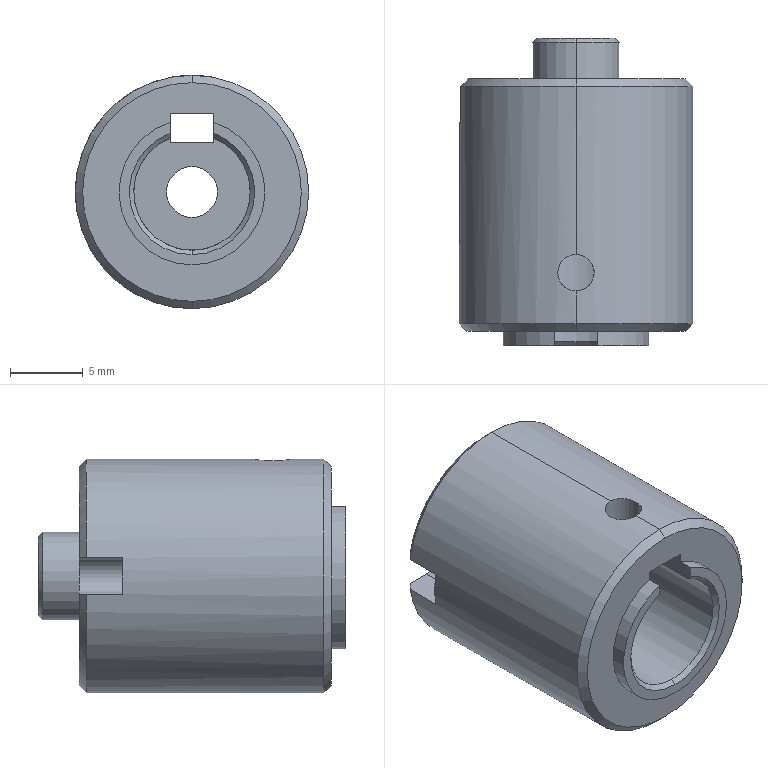Part | SolidWorks | features ICE 19, CirPattern 7, Chamfer 3, Extrusion 1, Fillet 1 | 1 solid | 35 faces | box 16 x 21.1 x 16 mm | volume 2636 mm3 | cylinder 12 | plane 12 | cone 11 | commonest cylinder face diameters 2.5 x3 3.5 x2 6 x2 10 x2 16 x2 8 x1
STEP:
#1=CARTESIAN_POINT('',(0.,4.8,2.7));
#2=VERTEX_POINT('',#1);
#3=CARTESIAN_POINT('',(0.,4.8,-2.7));
#4=VERTEX_POINT('',#3);
#5=CARTESIAN_POINT('',(0.,4.8,0.));
#6=DIRECTION('',(0.,1.,0.));
#7=DIRECTION('',(0.,0.,1.));
#8=AXIS2_PLACEMENT_3D('',#5,#6,#7);
#9=CIRCLE('',#8,2.7);
#10=EDGE_CURVE('',#2,#4,#9,.T.);
#11=ORIENTED_EDGE('',*,*,#10,.F.);
#12=CARTESIAN_POINT('',(0.,4.5,3.));
#13=VERTEX_POINT('',#12);
#14=CARTESIAN_POINT('',(0.,4.8,2.7));
#15=DIRECTION('',(0.,-0.7071,0.7071));
#16=VECTOR('',#15,1000.);
#17=LINE('',#14,#16);
#18=EDGE_CURVE('',#2,#13,#17,.T.);
#19=ORIENTED_EDGE('',*,*,#18,.T.);
#20=CARTESIAN_POINT('',(0.,4.5,-3.));
#21=VERTEX_POINT('',#20);
#22=CARTESIAN_POINT('',(0.,4.5,0.));
#23=DIRECTION('',(0.,-1.,0.));
#24=DIRECTION('',(0.,0.,1.));
#25=AXIS2_PLACEMENT_3D('',#22,#23,#24);
#26=CIRCLE('',#25,3.);
#27=EDGE_CURVE('',#21,#13,#26,.T.);
#28=ORIENTED_EDGE('',*,*,#27,.F.);
#29=CARTESIAN_POINT('',(0.,4.8,-2.7));
#30=DIRECTION('',(0.,-0.7071,-0.7071));
#31=VECTOR('',#30,1000.);
#32=LINE('',#29,#31);
#33=EDGE_CURVE('',#4,#21,#32,.T.);
#34=ORIENTED_EDGE('',*,*,#33,.F.);
#35=EDGE_LOOP('',(#11,#19,#28,#34));
#36=FACE_OUTER_BOUND('',#35,.T.);
#37=CARTESIAN_POINT('',(0.,4.8,0.));
#38=DIRECTION('',(0.,-1.,0.));
#39=DIRECTION('',(0.,0.,-1.));
#40=AXIS2_PLACEMENT_3D('',#37,#38,#39);
#41=CONICAL_SURFACE('',#40,2.7,0.7854);
#42=ADVANCED_FACE('',(#36),#41,.T.);
#43=CARTESIAN_POINT('',(0.,4.5,-1.75));
#44=VERTEX_POINT('',#43);
#45=CARTESIAN_POINT('',(0.,4.5,1.75));
#46=VERTEX_POINT('',#45);
#47=CARTESIAN_POINT('',(0.,4.5,0.));
#48=DIRECTION('',(0.,1.,0.));
#49=DIRECTION('',(0.,0.,1.));
#50=AXIS2_PLACEMENT_3D('',#47,#48,#49);
#51=CIRCLE('',#50,1.75);
#52=EDGE_CURVE('',#44,#46,#51,.T.);
#53=ORIENTED_EDGE('',*,*,#52,.F.);
#54=CARTESIAN_POINT('',(0.,4.8,-2.05));
#55=VERTEX_POINT('',#54);
#56=CARTESIAN_POINT('',(0.,4.5,-1.75));
#57=DIRECTION('',(0.,0.7071,-0.7071));
#58=VECTOR('',#57,1000.);
#59=LINE('',#56,#58);
#60=EDGE_CURVE('',#44,#55,#59,.T.);
#61=ORIENTED_EDGE('',*,*,#60,.T.);
#62=CARTESIAN_POINT('',(0.,4.8,2.05));
#63=VERTEX_POINT('',#62);
#64=CARTESIAN_POINT('',(0.,4.8,0.));
#65=DIRECTION('',(0.,-1.,0.));
#66=DIRECTION('',(0.,0.,1.));
#67=AXIS2_PLACEMENT_3D('',#64,#65,#66);
#68=CIRCLE('',#67,2.05);
#69=EDGE_CURVE('',#63,#55,#68,.T.);
#70=ORIENTED_EDGE('',*,*,#69,.F.);
#71=CARTESIAN_POINT('',(0.,4.5,1.75));
#72=DIRECTION('',(0.,0.7071,0.7071));
#73=VECTOR('',#72,1000.);
#74=LINE('',#71,#73);
#75=EDGE_CURVE('',#46,#63,#74,.T.);
#76=ORIENTED_EDGE('',*,*,#75,.F.);
#77=EDGE_LOOP('',(#53,#61,#70,#76));
#78=FACE_OUTER_BOUND('',#77,.T.);
#79=CARTESIAN_POINT('',(0.,4.5,0.));
#80=DIRECTION('',(0.,1.,0.));
#81=DIRECTION('',(0.,0.,1.));
#82=AXIS2_PLACEMENT_3D('',#79,#80,#81);
#83=CONICAL_SURFACE('',#82,1.75,0.7854);
#84=ADVANCED_FACE('',(#78),#83,.F.);
#85=CARTESIAN_POINT('',(0.,-16.,-4.));
#86=VERTEX_POINT('',#85);
#87=CARTESIAN_POINT('',(1.5,-16.,3.708));
#88=VERTEX_POINT('',#87);
#89=CARTESIAN_POINT('',(0.,-16.,0.));
#90=DIRECTION('',(0.,-1.,0.));
#91=DIRECTION('',(0.,0.,-1.));
#92=AXIS2_PLACEMENT_3D('',#89,#90,#91);
#93=CIRCLE('',#92,4.);
#94=EDGE_CURVE('',#86,#88,#93,.T.);
#95=ORIENTED_EDGE('',*,*,#94,.F.);
#96=CARTESIAN_POINT('',(0.,-16.3,-4.3));
#97=VERTEX_POINT('',#96);
#98=CARTESIAN_POINT('',(0.,-16.,-4.));
#99=DIRECTION('',(0.,-0.7071,-0.7071));
#100=VECTOR('',#99,1000.);
#101=LINE('',#98,#100);
#102=EDGE_CURVE('',#86,#97,#101,.T.);
#103=ORIENTED_EDGE('',*,*,#102,.T.);
#104=CARTESIAN_POINT('',(1.5,-16.3,4.03));
#105=VERTEX_POINT('',#104);
#106=CARTESIAN_POINT('',(0.,-16.3,0.));
#107=DIRECTION('',(0.,1.,0.));
#108=DIRECTION('',(0.,0.,-1.));
#109=AXIS2_PLACEMENT_3D('',#106,#107,#108);
#110=CIRCLE('',#109,4.3);
#111=EDGE_CURVE('',#105,#97,#110,.T.);
#112=ORIENTED_EDGE('',*,*,#111,.F.);
#113=CARTESIAN_POINT('',(1.5,-16.,3.708));
#114=CARTESIAN_POINT('',(1.5,-16.1,3.816));
#115=CARTESIAN_POINT('',(1.5,-16.2,3.923));
#116=CARTESIAN_POINT('',(1.5,-16.3,4.03));
#117=B_SPLINE_CURVE_WITH_KNOTS('',3,(#113,#114,#115,#116),.UNSPECIFIED.,.F.,.F.,(4,4),(0.,0.0004399),.UNSPECIFIED.);
#118=EDGE_CURVE('',#88,#105,#117,.T.);
#119=ORIENTED_EDGE('',*,*,#118,.F.);
#120=EDGE_LOOP('',(#95,#103,#112,#119));
#121=FACE_OUTER_BOUND('',#120,.T.);
#122=CARTESIAN_POINT('',(0.,-16.,0.));
#123=DIRECTION('',(0.,-1.,0.));
#124=DIRECTION('',(0.,0.,-1.));
#125=AXIS2_PLACEMENT_3D('',#122,#123,#124);
#126=CONICAL_SURFACE('',#125,4.,0.7854);
#127=ADVANCED_FACE('',(#121),#126,.F.);
#128=CARTESIAN_POINT('',(0.,-15.3,-7.5));
#129=VERTEX_POINT('',#128);
#130=CARTESIAN_POINT('',(0.,-15.3,7.5));
#131=VERTEX_POINT('',#130);
#132=CARTESIAN_POINT('',(0.,-15.3,0.));
#133=DIRECTION('',(0.,-1.,0.));
#134=DIRECTION('',(0.,0.,-1.));
#135=AXIS2_PLACEMENT_3D('',#132,#133,#134);
#136=CIRCLE('',#135,7.5);
#137=EDGE_CURVE('',#129,#131,#136,.T.);
#138=ORIENTED_EDGE('',*,*,#137,.F.);
#139=CARTESIAN_POINT('',(0.,-14.8,-8.));
#140=VERTEX_POINT('',#139);
#141=CARTESIAN_POINT('',(0.,-15.3,-7.5));
#142=DIRECTION('',(0.,0.7071,-0.7071));
#143=VECTOR('',#142,1000.);
#144=LINE('',#141,#143);
#145=EDGE_CURVE('',#129,#140,#144,.T.);
#146=ORIENTED_EDGE('',*,*,#145,.T.);
#147=CARTESIAN_POINT('',(0.,-14.8,8.));
#148=VERTEX_POINT('',#147);
#149=CARTESIAN_POINT('',(0.,-14.8,0.));
#150=DIRECTION('',(0.,1.,0.));
#151=DIRECTION('',(0.,0.,-1.));
#152=AXIS2_PLACEMENT_3D('',#149,#150,#151);
#153=CIRCLE('',#152,8.);
#154=EDGE_CURVE('',#148,#140,#153,.T.);
#155=ORIENTED_EDGE('',*,*,#154,.F.);
#156=CARTESIAN_POINT('',(0.,-15.3,7.5));
#157=DIRECTION('',(0.,0.7071,0.7071));
#158=VECTOR('',#157,1000.);
#159=LINE('',#156,#158);
#160=EDGE_CURVE('',#131,#148,#159,.T.);
#161=ORIENTED_EDGE('',*,*,#160,.F.);
#162=EDGE_LOOP('',(#138,#146,#155,#161));
#163=FACE_OUTER_BOUND('',#162,.T.);
#164=CARTESIAN_POINT('',(0.,-15.3,0.));
#165=DIRECTION('',(0.,1.,0.));
#166=DIRECTION('',(0.,0.,1.));
#167=AXIS2_PLACEMENT_3D('',#164,#165,#166);
#168=CONICAL_SURFACE('',#167,7.5,0.7854);
#169=ADVANCED_FACE('',(#163),#168,.T.);
#170=CARTESIAN_POINT('',(0.,2.,7.5));
#171=VERTEX_POINT('',#170);
#172=CARTESIAN_POINT('',(0.,2.,-7.5));
#173=VERTEX_POINT('',#172);
#174=CARTESIAN_POINT('',(0.,2.,0.));
#175=DIRECTION('',(0.,1.,0.));
#176=DIRECTION('',(0.,0.,1.));
#177=AXIS2_PLACEMENT_3D('',#174,#175,#176);
#178=CIRCLE('',#177,7.5);
#179=EDGE_CURVE('',#171,#173,#178,.T.);
#180=ORIENTED_EDGE('',*,*,#179,.F.);
#181=CARTESIAN_POINT('',(0.,1.5,8.));
#182=VERTEX_POINT('',#181);
#183=CARTESIAN_POINT('',(0.,2.,7.5));
#184=DIRECTION('',(0.,-0.7071,0.7071));
#185=VECTOR('',#184,1000.);
#186=LINE('',#183,#185);
#187=EDGE_CURVE('',#171,#182,#186,.T.);
#188=ORIENTED_EDGE('',*,*,#187,.T.);
#189=CARTESIAN_POINT('',(0.,1.5,-8.));
#190=VERTEX_POINT('',#189);
#191=CARTESIAN_POINT('',(0.,1.5,0.));
#192=DIRECTION('',(0.,-1.,0.));
#193=DIRECTION('',(0.,0.,1.));
#194=AXIS2_PLACEMENT_3D('',#191,#192,#193);
#195=CIRCLE('',#194,8.);
#196=EDGE_CURVE('',#190,#182,#195,.T.);
#197=ORIENTED_EDGE('',*,*,#196,.F.);
#198=CARTESIAN_POINT('',(0.,2.,-7.5));
#199=DIRECTION('',(0.,-0.7071,-0.7071));
#200=VECTOR('',#199,1000.);
#201=LINE('',#198,#200);
#202=EDGE_CURVE('',#173,#190,#201,.T.);
#203=ORIENTED_EDGE('',*,*,#202,.F.);
#204=EDGE_LOOP('',(#180,#188,#197,#203));
#205=FACE_OUTER_BOUND('',#204,.T.);
#206=CARTESIAN_POINT('',(0.,2.,0.));
#207=DIRECTION('',(0.,-1.,0.));
#208=DIRECTION('',(0.,0.,-1.));
#209=AXIS2_PLACEMENT_3D('',#206,#207,#208);
#210=CONICAL_SURFACE('',#209,7.5,0.7854);
#211=ADVANCED_FACE('',(#205),#210,.T.);
#212=CARTESIAN_POINT('',(-7.395,2.,-1.25));
#213=VERTEX_POINT('',#212);
#214=CARTESIAN_POINT('',(0.,2.,0.));
#215=DIRECTION('',(0.,1.,0.));
#216=DIRECTION('',(0.,0.,1.));
#217=AXIS2_PLACEMENT_3D('',#214,#215,#216);
#218=CIRCLE('',#217,7.5);
#219=EDGE_CURVE('',#173,#213,#218,.T.);
#220=ORIENTED_EDGE('',*,*,#219,.F.);
#221=ORIENTED_EDGE('',*,*,#202,.T.);
#222=CARTESIAN_POINT('',(-7.902,1.5,-1.25));
#223=VERTEX_POINT('',#222);
#224=CARTESIAN_POINT('',(0.,1.5,0.));
#225=DIRECTION('',(0.,-1.,0.));
#226=DIRECTION('',(0.,0.,1.));
#227=AXIS2_PLACEMENT_3D('',#224,#225,#226);
#228=CIRCLE('',#227,8.);
#229=EDGE_CURVE('',#223,#190,#228,.T.);
#230=ORIENTED_EDGE('',*,*,#229,.F.);
#231=CARTESIAN_POINT('',(-7.395,2.,-1.25));
#232=CARTESIAN_POINT('',(-7.564,1.833,-1.25));
#233=CARTESIAN_POINT('',(-7.733,1.667,-1.25));
#234=CARTESIAN_POINT('',(-7.902,1.5,-1.25));
#235=B_SPLINE_CURVE_WITH_KNOTS('',3,(#231,#232,#233,#234),.UNSPECIFIED.,.F.,.F.,(4,4),(0.,0.0007118),.UNSPECIFIED.);
#236=EDGE_CURVE('',#213,#223,#235,.T.);
#237=ORIENTED_EDGE('',*,*,#236,.F.);
#238=EDGE_LOOP('',(#220,#221,#230,#237));
#239=FACE_OUTER_BOUND('',#238,.T.);
#240=CARTESIAN_POINT('',(0.,2.,0.));
#241=DIRECTION('',(0.,-1.,0.));
#242=DIRECTION('',(0.,0.,-1.));
#243=AXIS2_PLACEMENT_3D('',#240,#241,#242);
#244=CONICAL_SURFACE('',#243,7.5,0.7854);
#245=ADVANCED_FACE('',(#239),#244,.T.);
#246=CARTESIAN_POINT('',(-1.25,-11.3,5.4));
#247=VERTEX_POINT('',#246);
#248=CARTESIAN_POINT('',(1.25,-11.3,5.4));
#249=VERTEX_POINT('',#248);
#250=CARTESIAN_POINT('',(0.,-11.3,5.4));
#251=DIRECTION('',(0.,0.,1.));
#252=DIRECTION('',(1.,0.,0.));
#253=AXIS2_PLACEMENT_3D('',#250,#251,#252);
#254=CIRCLE('',#253,1.25);
#255=EDGE_CURVE('',#247,#249,#254,.T.);
#256=ORIENTED_EDGE('',*,*,#255,.F.);
#257=CARTESIAN_POINT('',(-1.25,-11.3,7.902));
#258=VERTEX_POINT('',#257);
#259=CARTESIAN_POINT('',(-1.25,-11.3,3.));
#260=DIRECTION('',(0.,0.,1.));
#261=VECTOR('',#260,1000.);
#262=LINE('',#259,#261);
#263=EDGE_CURVE('',#247,#258,#262,.T.);
#264=ORIENTED_EDGE('',*,*,#263,.T.);
#265=CARTESIAN_POINT('',(0.,-12.55,8.));
#266=VERTEX_POINT('',#265);
#267=CARTESIAN_POINT('',(0.,-12.55,8.));
#268=CARTESIAN_POINT('',(-0.1655,-12.55,8.));
#269=CARTESIAN_POINT('',(-0.3279,-12.517,7.995));
#270=CARTESIAN_POINT('',(-0.6306,-12.392,7.977));
#271=CARTESIAN_POINT('',(-0.7691,-12.299,7.964));
#272=CARTESIAN_POINT('',(-0.9994,-12.068,7.938));
#273=CARTESIAN_POINT('',(-1.092,-11.929,7.925));
#274=CARTESIAN_POINT('',(-1.217,-11.628,7.907));
#275=CARTESIAN_POINT('',(-1.25,-11.463,7.902));
#276=CARTESIAN_POINT('',(-1.25,-11.3,7.902));
#277=B_SPLINE_CURVE_WITH_KNOTS('',3,(#267,#268,#269,#270,#271,#272,#273,#274,#275,#276),.UNSPECIFIED.,.F.,.F.,(4,2,2,2,4),(0.,0.0004894,0.0009788,0.001468,0.001958),.UNSPECIFIED.);
#278=EDGE_CURVE('',#266,#258,#277,.T.);
#279=ORIENTED_EDGE('',*,*,#278,.F.);
#280=CARTESIAN_POINT('',(1.25,-11.3,7.902));
#281=VERTEX_POINT('',#280);
#282=CARTESIAN_POINT('',(1.25,-11.3,7.902));
#283=CARTESIAN_POINT('',(1.25,-11.465,7.902));
#284=CARTESIAN_POINT('',(1.217,-11.628,7.907));
#285=CARTESIAN_POINT('',(1.092,-11.93,7.925));
#286=CARTESIAN_POINT('',(0.9992,-12.069,7.938));
#287=CARTESIAN_POINT('',(0.7692,-12.299,7.964));
#288=CARTESIAN_POINT('',(0.6301,-12.392,7.977));
#289=CARTESIAN_POINT('',(0.3296,-12.517,7.995));
#290=CARTESIAN_POINT('',(0.1653,-12.55,8.));
#291=CARTESIAN_POINT('',(0.,-12.55,8.));
#292=B_SPLINE_CURVE_WITH_KNOTS('',3,(#282,#283,#284,#285,#286,#287,#288,#289,#290,#291),.UNSPECIFIED.,.F.,.F.,(4,2,2,2,4),(0.005871,0.00636,0.006849,0.007338,0.007827),.UNSPECIFIED.);
#293=EDGE_CURVE('',#281,#266,#292,.T.);
#294=ORIENTED_EDGE('',*,*,#293,.F.);
#295=CARTESIAN_POINT('',(1.25,-11.3,3.));
#296=DIRECTION('',(0.,0.,1.));
#297=VECTOR('',#296,1000.);
#298=LINE('',#295,#297);
#299=EDGE_CURVE('',#249,#281,#298,.T.);
#300=ORIENTED_EDGE('',*,*,#299,.F.);
#301=EDGE_LOOP('',(#256,#264,#279,#294,#300));
#302=FACE_OUTER_BOUND('',#301,.T.);
#303=CARTESIAN_POINT('',(0.,-11.3,3.));
#304=DIRECTION('',(0.,0.,1.));
#305=DIRECTION('',(1.,0.,0.));
#306=AXIS2_PLACEMENT_3D('',#303,#304,#305);
#307=CYLINDRICAL_SURFACE('',#306,1.25);
#308=ADVANCED_FACE('',(#302),#307,.F.);
#309=ORIENTED_EDGE('',*,*,#27,.T.);
#310=CARTESIAN_POINT('',(0.,2.,3.));
#311=VERTEX_POINT('',#310);
#312=CARTESIAN_POINT('',(0.,4.8,3.));
#313=DIRECTION('',(0.,-1.,0.));
#314=VECTOR('',#313,1000.);
#315=LINE('',#312,#314);
#316=EDGE_CURVE('',#13,#311,#315,.T.);
#317=ORIENTED_EDGE('',*,*,#316,.T.);
#318=CARTESIAN_POINT('',(0.,2.,-3.));
#319=VERTEX_POINT('',#318);
#320=CARTESIAN_POINT('',(0.,2.,0.));
#321=DIRECTION('',(0.,1.,0.));
#322=DIRECTION('',(0.,0.,1.));
#323=AXIS2_PLACEMENT_3D('',#320,#321,#322);
#324=CIRCLE('',#323,3.);
#325=EDGE_CURVE('',#311,#319,#324,.T.);
#326=ORIENTED_EDGE('',*,*,#325,.T.);
#327=CARTESIAN_POINT('',(0.,4.8,-3.));
#328=DIRECTION('',(0.,-1.,0.));
#329=VECTOR('',#328,1000.);
#330=LINE('',#327,#329);
#331=EDGE_CURVE('',#21,#319,#330,.T.);
#332=ORIENTED_EDGE('',*,*,#331,.F.);
#333=EDGE_LOOP('',(#309,#317,#326,#332));
#334=FACE_OUTER_BOUND('',#333,.T.);
#335=CARTESIAN_POINT('',(0.,4.8,0.));
#336=DIRECTION('',(0.,-1.,0.));
#337=DIRECTION('',(0.,0.,-1.));
#338=AXIS2_PLACEMENT_3D('',#335,#336,#337);
#339=CYLINDRICAL_SURFACE('',#338,3.);
#340=ADVANCED_FACE('',(#334),#339,.T.);
#341=ORIENTED_EDGE('',*,*,#52,.T.);
#342=CARTESIAN_POINT('',(0.,0.,1.75));
#343=VERTEX_POINT('',#342);
#344=CARTESIAN_POINT('',(0.,2.,1.75));
#345=DIRECTION('',(0.,-1.,0.));
#346=VECTOR('',#345,1000.);
#347=LINE('',#344,#346);
#348=EDGE_CURVE('',#46,#343,#347,.T.);
#349=ORIENTED_EDGE('',*,*,#348,.T.);
#350=CARTESIAN_POINT('',(0.,0.,-1.75));
#351=VERTEX_POINT('',#350);
#352=CARTESIAN_POINT('',(0.,0.,0.));
#353=DIRECTION('',(0.,1.,0.));
#354=DIRECTION('',(0.,0.,1.));
#355=AXIS2_PLACEMENT_3D('',#352,#353,#354);
#356=CIRCLE('',#355,1.75);
#357=EDGE_CURVE('',#351,#343,#356,.T.);
#358=ORIENTED_EDGE('',*,*,#357,.F.);
#359=CARTESIAN_POINT('',(0.,2.,-1.75));
#360=DIRECTION('',(0.,-1.,0.));
#361=VECTOR('',#360,1000.);
#362=LINE('',#359,#361);
#363=EDGE_CURVE('',#44,#351,#362,.T.);
#364=ORIENTED_EDGE('',*,*,#363,.F.);
#365=EDGE_LOOP('',(#341,#349,#358,#364));
#366=FACE_OUTER_BOUND('',#365,.T.);
#367=CARTESIAN_POINT('',(0.,2.,0.));
#368=DIRECTION('',(0.,-1.,0.));
#369=DIRECTION('',(0.,0.,-1.));
#370=AXIS2_PLACEMENT_3D('',#367,#368,#369);
#371=CYLINDRICAL_SURFACE('',#370,1.75);
#372=ADVANCED_FACE('',(#366),#371,.F.);
#373=CARTESIAN_POINT('',(-1.5,-15.3,4.77));
#374=VERTEX_POINT('',#373);
#375=CARTESIAN_POINT('',(0.,-15.3,-5.));
#376=VERTEX_POINT('',#375);
#377=CARTESIAN_POINT('',(0.,-15.3,0.));
#378=DIRECTION('',(0.,-1.,0.));
#379=DIRECTION('',(0.,0.,-1.));
#380=AXIS2_PLACEMENT_3D('',#377,#378,#379);
#381=CIRCLE('',#380,5.);
#382=EDGE_CURVE('',#374,#376,#381,.T.);
#383=ORIENTED_EDGE('',*,*,#382,.T.);
#384=CARTESIAN_POINT('',(0.,-16.3,-5.));
#385=VERTEX_POINT('',#384);
#386=CARTESIAN_POINT('',(0.,-15.3,-5.));
#387=DIRECTION('',(0.,-1.,0.));
#388=VECTOR('',#387,1000.);
#389=LINE('',#386,#388);
#390=EDGE_CURVE('',#376,#385,#389,.T.);
#391=ORIENTED_EDGE('',*,*,#390,.T.);
#392=CARTESIAN_POINT('',(-1.5,-16.3,4.77));
#393=VERTEX_POINT('',#392);
#394=CARTESIAN_POINT('',(0.,-16.3,0.));
#395=DIRECTION('',(0.,-1.,0.));
#396=DIRECTION('',(0.,0.,-1.));
#397=AXIS2_PLACEMENT_3D('',#394,#395,#396);
#398=CIRCLE('',#397,5.);
#399=EDGE_CURVE('',#393,#385,#398,.T.);
#400=ORIENTED_EDGE('',*,*,#399,.F.);
#401=CARTESIAN_POINT('',(-1.5,-15.3,4.77));
#402=DIRECTION('',(0.,-1.,0.));
#403=VECTOR('',#402,1000.);
#404=LINE('',#401,#403);
#405=EDGE_CURVE('',#374,#393,#404,.T.);
#406=ORIENTED_EDGE('',*,*,#405,.F.);
#407=EDGE_LOOP('',(#383,#391,#400,#406));
#408=FACE_OUTER_BOUND('',#407,.T.);
#409=CARTESIAN_POINT('',(0.,-15.3,0.));
#410=DIRECTION('',(0.,-1.,0.));
#411=DIRECTION('',(0.,0.,-1.));
#412=AXIS2_PLACEMENT_3D('',#409,#410,#411);
#413=CYLINDRICAL_SURFACE('',#412,5.);
#414=ADVANCED_FACE('',(#408),#413,.T.);
#415=ORIENTED_EDGE('',*,*,#154,.T.);
#416=CARTESIAN_POINT('',(0.,-16.3,-8.));
#417=DIRECTION('',(0.,1.,0.));
#418=VECTOR('',#417,1000.);
#419=LINE('',#416,#418);
#420=EDGE_CURVE('',#140,#190,#419,.T.);
#421=ORIENTED_EDGE('',*,*,#420,.T.);
#422=ORIENTED_EDGE('',*,*,#196,.T.);
#423=CARTESIAN_POINT('',(0.,-10.05,8.));
#424=VERTEX_POINT('',#423);
#425=CARTESIAN_POINT('',(0.,-16.3,8.));
#426=DIRECTION('',(0.,1.,0.));
#427=VECTOR('',#426,1000.);
#428=LINE('',#425,#427);
#429=EDGE_CURVE('',#424,#182,#428,.T.);
#430=ORIENTED_EDGE('',*,*,#429,.F.);
#431=CARTESIAN_POINT('',(0.,-10.05,8.));
#432=CARTESIAN_POINT('',(0.1633,-10.05,8.));
#433=CARTESIAN_POINT('',(0.3281,-10.083,7.995));
#434=CARTESIAN_POINT('',(0.6291,-10.208,7.977));
#435=CARTESIAN_POINT('',(0.7683,-10.301,7.964));
#436=CARTESIAN_POINT('',(0.9412,-10.473,7.945));
#437=CARTESIAN_POINT('',(0.994,-10.538,7.938));
#438=CARTESIAN_POINT('',(1.085,-10.673,7.926));
#439=CARTESIAN_POINT('',(1.123,-10.745,7.921));
#440=CARTESIAN_POINT('',(1.217,-10.972,7.907));
#441=CARTESIAN_POINT('',(1.25,-11.135,7.902));
#442=CARTESIAN_POINT('',(1.25,-11.3,7.902));
#443=B_SPLINE_CURVE_WITH_KNOTS('',3,(#431,#432,#433,#434,#435,#436,#437,#438,#439,#440,#441,#442),.UNSPECIFIED.,.F.,.F.,(4,2,2,2,2,4),(0.003914,0.004403,0.004893,0.005137,0.005382,0.005871),.UNSPECIFIED.);
#444=EDGE_CURVE('',#424,#281,#443,.T.);
#445=ORIENTED_EDGE('',*,*,#444,.T.);
#446=ORIENTED_EDGE('',*,*,#293,.T.);
#447=CARTESIAN_POINT('',(0.,-16.3,8.));
#448=DIRECTION('',(0.,1.,0.));
#449=VECTOR('',#448,1000.);
#450=LINE('',#447,#449);
#451=EDGE_CURVE('',#148,#266,#450,.T.);
#452=ORIENTED_EDGE('',*,*,#451,.F.);
#453=EDGE_LOOP('',(#415,#421,#422,#430,#445,#446,#452));
#454=FACE_OUTER_BOUND('',#453,.T.);
#455=CARTESIAN_POINT('',(0.,-16.3,0.));
#456=DIRECTION('',(0.,1.,0.));
#457=DIRECTION('',(0.,0.,1.));
#458=AXIS2_PLACEMENT_3D('',#455,#456,#457);
#459=CYLINDRICAL_SURFACE('',#458,8.);
#460=ADVANCED_FACE('',(#454),#459,.T.);
#461=CARTESIAN_POINT('',(-1.5,2.,3.4));
#462=VERTEX_POINT('',#461);
#463=CARTESIAN_POINT('',(-1.5,2.,5.4));
#464=VERTEX_POINT('',#463);
#465=CARTESIAN_POINT('',(-1.5,2.,0.));
#466=DIRECTION('',(0.,0.,1.));
#467=VECTOR('',#466,1000.);
#468=LINE('',#465,#467);
#469=EDGE_CURVE('',#462,#464,#468,.T.);
#470=ORIENTED_EDGE('',*,*,#469,.F.);
#471=CARTESIAN_POINT('',(1.5,2.,3.4));
#472=VERTEX_POINT('',#471);
#473=CARTESIAN_POINT('',(0.,2.,3.4));
#474=DIRECTION('',(-1.,0.,0.));
#475=VECTOR('',#474,1000.);
#476=LINE('',#473,#475);
#477=EDGE_CURVE('',#472,#462,#476,.T.);
#478=ORIENTED_EDGE('',*,*,#477,.F.);
#479=CARTESIAN_POINT('',(1.5,2.,5.4));
#480=VERTEX_POINT('',#479);
#481=CARTESIAN_POINT('',(1.5,2.,0.));
#482=DIRECTION('',(0.,0.,-1.));
#483=VECTOR('',#482,1000.);
#484=LINE('',#481,#483);
#485=EDGE_CURVE('',#480,#472,#484,.T.);
#486=ORIENTED_EDGE('',*,*,#485,.F.);
#487=CARTESIAN_POINT('',(0.,2.,5.4));
#488=DIRECTION('',(1.,0.,0.));
#489=VECTOR('',#488,1000.);
#490=LINE('',#487,#489);
#491=EDGE_CURVE('',#464,#480,#490,.T.);
#492=ORIENTED_EDGE('',*,*,#491,.F.);
#493=EDGE_LOOP('',(#470,#478,#486,#492));
#494=FACE_BOUND('',#493,.T.);
#495=CARTESIAN_POINT('',(-7.395,2.,1.25));
#496=VERTEX_POINT('',#495);
#497=CARTESIAN_POINT('',(-5.8,2.,1.25));
#498=VERTEX_POINT('',#497);
#499=CARTESIAN_POINT('',(-9.,2.,1.25));
#500=DIRECTION('',(1.,0.,0.));
#501=VECTOR('',#500,1000.);
#502=LINE('',#499,#501);
#503=EDGE_CURVE('',#496,#498,#502,.T.);
#504=ORIENTED_EDGE('',*,*,#503,.F.);
#505=CARTESIAN_POINT('',(0.,2.,0.));
#506=DIRECTION('',(0.,1.,0.));
#507=DIRECTION('',(0.,0.,1.));
#508=AXIS2_PLACEMENT_3D('',#505,#506,#507);
#509=CIRCLE('',#508,7.5);
#510=EDGE_CURVE('',#496,#171,#509,.T.);
#511=ORIENTED_EDGE('',*,*,#510,.T.);
#512=ORIENTED_EDGE('',*,*,#179,.T.);
#513=ORIENTED_EDGE('',*,*,#219,.T.);
#514=CARTESIAN_POINT('',(-5.8,2.,-1.25));
#515=VERTEX_POINT('',#514);
#516=CARTESIAN_POINT('',(-9.,2.,-1.25));
#517=DIRECTION('',(-1.,0.,0.));
#518=VECTOR('',#517,1000.);
#519=LINE('',#516,#518);
#520=EDGE_CURVE('',#515,#213,#519,.T.);
#521=ORIENTED_EDGE('',*,*,#520,.F.);
#522=CARTESIAN_POINT('',(-5.8,2.,0.));
#523=DIRECTION('',(0.,1.,0.));
#524=DIRECTION('',(0.,0.,-1.));
#525=AXIS2_PLACEMENT_3D('',#522,#523,#524);
#526=CIRCLE('',#525,1.25);
#527=EDGE_CURVE('',#498,#515,#526,.T.);
#528=ORIENTED_EDGE('',*,*,#527,.F.);
#529=EDGE_LOOP('',(#504,#511,#512,#513,#521,#528));
#530=FACE_OUTER_BOUND('',#529,.T.);
#531=CARTESIAN_POINT('',(0.,2.,0.));
#532=DIRECTION('',(0.,1.,0.));
#533=DIRECTION('',(0.,0.,1.));
#534=AXIS2_PLACEMENT_3D('',#531,#532,#533);
#535=CIRCLE('',#534,3.);
#536=EDGE_CURVE('',#319,#311,#535,.T.);
#537=ORIENTED_EDGE('',*,*,#536,.F.);
#538=ORIENTED_EDGE('',*,*,#325,.F.);
#539=EDGE_LOOP('',(#537,#538));
#540=FACE_BOUND('',#539,.T.);
#541=CARTESIAN_POINT('',(0.,2.,0.));
#542=DIRECTION('',(0.,1.,0.));
#543=DIRECTION('',(0.,0.,1.));
#544=AXIS2_PLACEMENT_3D('',#541,#542,#543);
#545=PLANE('',#544);
#546=ADVANCED_FACE('',(#494,#530,#540),#545,.T.);
#547=CARTESIAN_POINT('',(1.5,-16.3,4.77));
#548=VERTEX_POINT('',#547);
#549=CARTESIAN_POINT('',(1.5,-16.3,5.4));
#550=DIRECTION('',(0.,0.,1.));
#551=VECTOR('',#550,1000.);
#552=LINE('',#549,#551);
#553=EDGE_CURVE('',#105,#548,#552,.T.);
#554=ORIENTED_EDGE('',*,*,#553,.F.);
#555=ORIENTED_EDGE('',*,*,#111,.T.);
#556=CARTESIAN_POINT('',(-1.5,-16.3,4.03));
#557=VERTEX_POINT('',#556);
#558=CARTESIAN_POINT('',(0.,-16.3,0.));
#559=DIRECTION('',(0.,1.,0.));
#560=DIRECTION('',(0.,0.,-1.));
#561=AXIS2_PLACEMENT_3D('',#558,#559,#560);
#562=CIRCLE('',#561,4.3);
#563=EDGE_CURVE('',#97,#557,#562,.T.);
#564=ORIENTED_EDGE('',*,*,#563,.T.);
#565=CARTESIAN_POINT('',(-1.5,-16.3,5.4));
#566=DIRECTION('',(0.,0.,-1.));
#567=VECTOR('',#566,1000.);
#568=LINE('',#565,#567);
#569=EDGE_CURVE('',#393,#557,#568,.T.);
#570=ORIENTED_EDGE('',*,*,#569,.F.);
#571=ORIENTED_EDGE('',*,*,#399,.T.);
#572=CARTESIAN_POINT('',(0.,-16.3,0.));
#573=DIRECTION('',(0.,-1.,0.));
#574=DIRECTION('',(0.,0.,-1.));
#575=AXIS2_PLACEMENT_3D('',#572,#573,#574);
#576=CIRCLE('',#575,5.);
#577=EDGE_CURVE('',#385,#548,#576,.T.);
#578=ORIENTED_EDGE('',*,*,#577,.T.);
#579=EDGE_LOOP('',(#554,#555,#564,#570,#571,#578));
#580=FACE_OUTER_BOUND('',#579,.T.);
#581=CARTESIAN_POINT('',(0.,-16.3,0.));
#582=DIRECTION('',(0.,-1.,0.));
#583=DIRECTION('',(0.,0.,-1.));
#584=AXIS2_PLACEMENT_3D('',#581,#582,#583);
#585=PLANE('',#584);
#586=ADVANCED_FACE('',(#580),#585,.T.);
#587=ORIENTED_EDGE('',*,*,#420,.F.);
#588=CARTESIAN_POINT('',(0.,-14.8,0.));
#589=DIRECTION('',(0.,1.,0.));
#590=DIRECTION('',(0.,0.,-1.));
#591=AXIS2_PLACEMENT_3D('',#588,#589,#590);
#592=CIRCLE('',#591,8.);
#593=EDGE_CURVE('',#140,#148,#592,.T.);
#594=ORIENTED_EDGE('',*,*,#593,.T.);
#595=ORIENTED_EDGE('',*,*,#451,.T.);
#596=ORIENTED_EDGE('',*,*,#278,.T.);
#597=CARTESIAN_POINT('',(-1.25,-11.3,7.902));
#598=CARTESIAN_POINT('',(-1.25,-11.218,7.902));
#599=CARTESIAN_POINT('',(-1.242,-11.135,7.903));
#600=CARTESIAN_POINT('',(-1.21,-10.975,7.908));
#601=CARTESIAN_POINT('',(-1.186,-10.897,7.912));
#602=CARTESIAN_POINT('',(-1.092,-10.67,7.925));
#603=CARTESIAN_POINT('',(-1.,-10.532,7.938));
#604=CARTESIAN_POINT('',(-0.7673,-10.3,7.964));
#605=CARTESIAN_POINT('',(-0.6297,-10.208,7.977));
#606=CARTESIAN_POINT('',(-0.4029,-10.114,7.99));
#607=CARTESIAN_POINT('',(-0.325,-10.09,7.994));
#608=CARTESIAN_POINT('',(-0.1645,-10.058,7.999));
#609=CARTESIAN_POINT('',(-0.08163,-10.05,8.));
#610=CARTESIAN_POINT('',(0.,-10.05,8.));
#611=B_SPLINE_CURVE_WITH_KNOTS('',3,(#597,#598,#599,#600,#601,#602,#603,#604,#605,#606,#607,#608,#609,#610),.UNSPECIFIED.,.F.,.F.,(4,2,2,2,2,2,4),(0.001958,0.002202,0.002447,0.002936,0.003425,0.003669,0.003914),.UNSPECIFIED.);
#612=EDGE_CURVE('',#258,#424,#611,.T.);
#613=ORIENTED_EDGE('',*,*,#612,.T.);
#614=ORIENTED_EDGE('',*,*,#429,.T.);
#615=CARTESIAN_POINT('',(-7.902,1.5,1.25));
#616=VERTEX_POINT('',#615);
#617=CARTESIAN_POINT('',(0.,1.5,0.));
#618=DIRECTION('',(0.,-1.,0.));
#619=DIRECTION('',(0.,0.,1.));
#620=AXIS2_PLACEMENT_3D('',#617,#618,#619);
#621=CIRCLE('',#620,8.);
#622=EDGE_CURVE('',#182,#616,#621,.T.);
#623=ORIENTED_EDGE('',*,*,#622,.T.);
#624=CARTESIAN_POINT('',(-7.902,-1.,1.25));
#625=VERTEX_POINT('',#624);
#626=CARTESIAN_POINT('',(-7.902,-16.3,1.25));
#627=DIRECTION('',(0.,-1.,0.));
#628=VECTOR('',#627,1000.);
#629=LINE('',#626,#628);
#630=EDGE_CURVE('',#616,#625,#629,.T.);
#631=ORIENTED_EDGE('',*,*,#630,.T.);
#632=CARTESIAN_POINT('',(-7.902,-1.,-1.25));
#633=VERTEX_POINT('',#632);
#634=CARTESIAN_POINT('',(0.,-1.,0.));
#635=DIRECTION('',(0.,-1.,0.));
#636=DIRECTION('',(0.,0.,-1.));
#637=AXIS2_PLACEMENT_3D('',#634,#635,#636);
#638=CIRCLE('',#637,8.);
#639=EDGE_CURVE('',#625,#633,#638,.T.);
#640=ORIENTED_EDGE('',*,*,#639,.T.);
#641=CARTESIAN_POINT('',(-7.902,-16.3,-1.25));
#642=DIRECTION('',(0.,1.,0.));
#643=VECTOR('',#642,1000.);
#644=LINE('',#641,#643);
#645=EDGE_CURVE('',#633,#223,#644,.T.);
#646=ORIENTED_EDGE('',*,*,#645,.T.);
#647=ORIENTED_EDGE('',*,*,#229,.T.);
#648=EDGE_LOOP('',(#587,#594,#595,#596,#613,#614,#623,#631,#640,#646,#647));
#649=FACE_OUTER_BOUND('',#648,.T.);
#650=CARTESIAN_POINT('',(0.,-16.3,0.));
#651=DIRECTION('',(0.,1.,0.));
#652=DIRECTION('',(0.,0.,1.));
#653=AXIS2_PLACEMENT_3D('',#650,#651,#652);
#654=CYLINDRICAL_SURFACE('',#653,8.);
#655=ADVANCED_FACE('',(#649),#654,.T.);
#656=CARTESIAN_POINT('',(-1.5,0.,3.708));
#657=VERTEX_POINT('',#656);
#658=CARTESIAN_POINT('',(-1.5,-16.,3.708));
#659=VERTEX_POINT('',#658);
#660=CARTESIAN_POINT('',(-1.5,0.,3.708));
#661=DIRECTION('',(0.,-1.,0.));
#662=VECTOR('',#661,1000.);
#663=LINE('',#660,#662);
#664=EDGE_CURVE('',#657,#659,#663,.T.);
#665=ORIENTED_EDGE('',*,*,#664,.T.);
#666=CARTESIAN_POINT('',(0.,-16.,0.));
#667=DIRECTION('',(0.,-1.,0.));
#668=DIRECTION('',(0.,0.,-1.));
#669=AXIS2_PLACEMENT_3D('',#666,#667,#668);
#670=CIRCLE('',#669,4.);
#671=EDGE_CURVE('',#659,#86,#670,.T.);
#672=ORIENTED_EDGE('',*,*,#671,.T.);
#673=ORIENTED_EDGE('',*,*,#94,.T.);
#674=CARTESIAN_POINT('',(1.5,0.,3.708));
#675=VERTEX_POINT('',#674);
#676=CARTESIAN_POINT('',(1.5,0.,3.708));
#677=DIRECTION('',(0.,1.,0.));
#678=VECTOR('',#677,1000.);
#679=LINE('',#676,#678);
#680=EDGE_CURVE('',#88,#675,#679,.T.);
#681=ORIENTED_EDGE('',*,*,#680,.T.);
#682=CARTESIAN_POINT('',(0.,0.,0.));
#683=DIRECTION('',(0.,-1.,0.));
#684=DIRECTION('',(0.,0.,1.));
#685=AXIS2_PLACEMENT_3D('',#682,#683,#684);
#686=CIRCLE('',#685,4.);
#687=EDGE_CURVE('',#657,#675,#686,.T.);
#688=ORIENTED_EDGE('',*,*,#687,.F.);
#689=EDGE_LOOP('',(#665,#672,#673,#681,#688));
#690=FACE_OUTER_BOUND('',#689,.T.);
#691=CARTESIAN_POINT('',(0.,0.,0.));
#692=DIRECTION('',(0.,1.,0.));
#693=DIRECTION('',(0.,0.,1.));
#694=AXIS2_PLACEMENT_3D('',#691,#692,#693);
#695=CYLINDRICAL_SURFACE('',#694,4.);
#696=ADVANCED_FACE('',(#690),#695,.F.);
#697=CARTESIAN_POINT('',(0.,-15.3,0.));
#698=DIRECTION('',(0.,-1.,0.));
#699=DIRECTION('',(0.,0.,-1.));
#700=AXIS2_PLACEMENT_3D('',#697,#698,#699);
#701=CIRCLE('',#700,7.5);
#702=EDGE_CURVE('',#131,#129,#701,.T.);
#703=ORIENTED_EDGE('',*,*,#702,.T.);
#704=ORIENTED_EDGE('',*,*,#137,.T.);
#705=EDGE_LOOP('',(#703,#704));
#706=FACE_OUTER_BOUND('',#705,.T.);
#707=CARTESIAN_POINT('',(1.5,-15.3,4.77));
#708=VERTEX_POINT('',#707);
#709=CARTESIAN_POINT('',(1.5,-15.3,5.4));
#710=VERTEX_POINT('',#709);
#711=CARTESIAN_POINT('',(1.5,-15.3,0.));
#712=DIRECTION('',(0.,0.,1.));
#713=VECTOR('',#712,1000.);
#714=LINE('',#711,#713);
#715=EDGE_CURVE('',#708,#710,#714,.T.);
#716=ORIENTED_EDGE('',*,*,#715,.F.);
#717=CARTESIAN_POINT('',(0.,-15.3,0.));
#718=DIRECTION('',(0.,-1.,0.));
#719=DIRECTION('',(0.,0.,-1.));
#720=AXIS2_PLACEMENT_3D('',#717,#718,#719);
#721=CIRCLE('',#720,5.);
#722=EDGE_CURVE('',#376,#708,#721,.T.);
#723=ORIENTED_EDGE('',*,*,#722,.F.);
#724=ORIENTED_EDGE('',*,*,#382,.F.);
#725=CARTESIAN_POINT('',(-1.5,-15.3,5.4));
#726=VERTEX_POINT('',#725);
#727=CARTESIAN_POINT('',(-1.5,-15.3,0.));
#728=DIRECTION('',(0.,0.,-1.));
#729=VECTOR('',#728,1000.);
#730=LINE('',#727,#729);
#731=EDGE_CURVE('',#726,#374,#730,.T.);
#732=ORIENTED_EDGE('',*,*,#731,.F.);
#733=CARTESIAN_POINT('',(0.,-15.3,5.4));
#734=DIRECTION('',(-1.,0.,0.));
#735=VECTOR('',#734,1000.);
#736=LINE('',#733,#735);
#737=EDGE_CURVE('',#710,#726,#736,.T.);
#738=ORIENTED_EDGE('',*,*,#737,.F.);
#739=EDGE_LOOP('',(#716,#723,#724,#732,#738));
#740=FACE_BOUND('',#739,.T.);
#741=CARTESIAN_POINT('',(0.,-15.3,0.));
#742=DIRECTION('',(0.,-1.,0.));
#743=DIRECTION('',(0.,0.,-1.));
#744=AXIS2_PLACEMENT_3D('',#741,#742,#743);
#745=PLANE('',#744);
#746=ADVANCED_FACE('',(#706,#740),#745,.T.);
#747=ORIENTED_EDGE('',*,*,#390,.F.);
#748=ORIENTED_EDGE('',*,*,#722,.T.);
#749=CARTESIAN_POINT('',(1.5,-15.3,4.77));
#750=DIRECTION('',(0.,1.,0.));
#751=VECTOR('',#750,1000.);
#752=LINE('',#749,#751);
#753=EDGE_CURVE('',#548,#708,#752,.T.);
#754=ORIENTED_EDGE('',*,*,#753,.F.);
#755=ORIENTED_EDGE('',*,*,#577,.F.);
#756=EDGE_LOOP('',(#747,#748,#754,#755));
#757=FACE_OUTER_BOUND('',#756,.T.);
#758=CARTESIAN_POINT('',(0.,-15.3,0.));
#759=DIRECTION('',(0.,-1.,0.));
#760=DIRECTION('',(0.,0.,-1.));
#761=AXIS2_PLACEMENT_3D('',#758,#759,#760);
#762=CYLINDRICAL_SURFACE('',#761,5.);
#763=ADVANCED_FACE('',(#757),#762,.T.);
#764=ORIENTED_EDGE('',*,*,#680,.F.);
#765=ORIENTED_EDGE('',*,*,#118,.T.);
#766=ORIENTED_EDGE('',*,*,#553,.T.);
#767=ORIENTED_EDGE('',*,*,#753,.T.);
#768=ORIENTED_EDGE('',*,*,#715,.T.);
#769=CARTESIAN_POINT('',(1.5,5.8,5.4));
#770=DIRECTION('',(0.,-1.,0.));
#771=VECTOR('',#770,1000.);
#772=LINE('',#769,#771);
#773=EDGE_CURVE('',#480,#710,#772,.T.);
#774=ORIENTED_EDGE('',*,*,#773,.F.);
#775=ORIENTED_EDGE('',*,*,#485,.T.);
#776=CARTESIAN_POINT('',(1.5,0.,3.4));
#777=VERTEX_POINT('',#776);
#778=CARTESIAN_POINT('',(1.5,4.8,3.4));
#779=DIRECTION('',(0.,-1.,0.));
#780=VECTOR('',#779,1000.);
#781=LINE('',#778,#780);
#782=EDGE_CURVE('',#472,#777,#781,.T.);
#783=ORIENTED_EDGE('',*,*,#782,.T.);
#784=CARTESIAN_POINT('',(1.5,0.,0.));
#785=DIRECTION('',(0.,0.,-1.));
#786=VECTOR('',#785,1000.);
#787=LINE('',#784,#786);
#788=EDGE_CURVE('',#675,#777,#787,.T.);
#789=ORIENTED_EDGE('',*,*,#788,.F.);
#790=EDGE_LOOP('',(#764,#765,#766,#767,#768,#774,#775,#783,#789));
#791=FACE_OUTER_BOUND('',#790,.T.);
#792=CARTESIAN_POINT('',(1.5,5.8,5.4));
#793=DIRECTION('',(1.,0.,0.));
#794=DIRECTION('',(0.,0.,-1.));
#795=AXIS2_PLACEMENT_3D('',#792,#793,#794);
#796=PLANE('',#795);
#797=ADVANCED_FACE('',(#791),#796,.F.);
#798=ORIENTED_EDGE('',*,*,#569,.T.);
#799=CARTESIAN_POINT('',(-1.5,-16.3,4.03));
#800=CARTESIAN_POINT('',(-1.5,-16.2,3.923));
#801=CARTESIAN_POINT('',(-1.5,-16.1,3.816));
#802=CARTESIAN_POINT('',(-1.5,-16.,3.708));
#803=B_SPLINE_CURVE_WITH_KNOTS('',3,(#799,#800,#801,#802),.UNSPECIFIED.,.F.,.F.,(4,4),(0.,0.0004399),.UNSPECIFIED.);
#804=EDGE_CURVE('',#557,#659,#803,.T.);
#805=ORIENTED_EDGE('',*,*,#804,.T.);
#806=ORIENTED_EDGE('',*,*,#664,.F.);
#807=CARTESIAN_POINT('',(-1.5,0.,3.4));
#808=VERTEX_POINT('',#807);
#809=CARTESIAN_POINT('',(-1.5,0.,0.));
#810=DIRECTION('',(0.,0.,1.));
#811=VECTOR('',#810,1000.);
#812=LINE('',#809,#811);
#813=EDGE_CURVE('',#808,#657,#812,.T.);
#814=ORIENTED_EDGE('',*,*,#813,.F.);
#815=CARTESIAN_POINT('',(-1.5,4.8,3.4));
#816=DIRECTION('',(0.,-1.,0.));
#817=VECTOR('',#816,1000.);
#818=LINE('',#815,#817);
#819=EDGE_CURVE('',#462,#808,#818,.T.);
#820=ORIENTED_EDGE('',*,*,#819,.F.);
#821=ORIENTED_EDGE('',*,*,#469,.T.);
#822=CARTESIAN_POINT('',(-1.5,5.8,5.4));
#823=DIRECTION('',(0.,-1.,0.));
#824=VECTOR('',#823,1000.);
#825=LINE('',#822,#824);
#826=EDGE_CURVE('',#464,#726,#825,.T.);
#827=ORIENTED_EDGE('',*,*,#826,.T.);
#828=ORIENTED_EDGE('',*,*,#731,.T.);
#829=ORIENTED_EDGE('',*,*,#405,.T.);
#830=EDGE_LOOP('',(#798,#805,#806,#814,#820,#821,#827,#828,#829));
#831=FACE_OUTER_BOUND('',#830,.T.);
#832=CARTESIAN_POINT('',(-1.5,5.8,5.4));
#833=DIRECTION('',(-1.,0.,0.));
#834=DIRECTION('',(0.,0.,1.));
#835=AXIS2_PLACEMENT_3D('',#832,#833,#834);
#836=PLANE('',#835);
#837=ADVANCED_FACE('',(#831),#836,.F.);
#838=CARTESIAN_POINT('',(0.,-11.3,5.4));
#839=DIRECTION('',(0.,0.,1.));
#840=DIRECTION('',(1.,0.,0.));
#841=AXIS2_PLACEMENT_3D('',#838,#839,#840);
#842=CIRCLE('',#841,1.25);
#843=EDGE_CURVE('',#249,#247,#842,.T.);
#844=ORIENTED_EDGE('',*,*,#843,.T.);
#845=ORIENTED_EDGE('',*,*,#255,.T.);
#846=EDGE_LOOP('',(#844,#845));
#847=FACE_BOUND('',#846,.T.);
#848=ORIENTED_EDGE('',*,*,#826,.F.);
#849=ORIENTED_EDGE('',*,*,#491,.T.);
#850=ORIENTED_EDGE('',*,*,#773,.T.);
#851=ORIENTED_EDGE('',*,*,#737,.T.);
#852=EDGE_LOOP('',(#848,#849,#850,#851));
#853=FACE_OUTER_BOUND('',#852,.T.);
#854=CARTESIAN_POINT('',(-1.5,5.8,5.4));
#855=DIRECTION('',(0.,0.,1.));
#856=DIRECTION('',(1.,0.,0.));
#857=AXIS2_PLACEMENT_3D('',#854,#855,#856);
#858=PLANE('',#857);
#859=ADVANCED_FACE('',(#847,#853),#858,.F.);
#860=ORIENTED_EDGE('',*,*,#357,.T.);
#861=CARTESIAN_POINT('',(0.,0.,0.));
#862=DIRECTION('',(0.,1.,0.));
#863=DIRECTION('',(0.,0.,1.));
#864=AXIS2_PLACEMENT_3D('',#861,#862,#863);
#865=CIRCLE('',#864,1.75);
#866=EDGE_CURVE('',#343,#351,#865,.T.);
#867=ORIENTED_EDGE('',*,*,#866,.T.);
#868=EDGE_LOOP('',(#860,#867));
#869=FACE_BOUND('',#868,.T.);
#870=CARTESIAN_POINT('',(0.,0.,3.4));
#871=DIRECTION('',(-1.,0.,0.));
#872=VECTOR('',#871,1000.);
#873=LINE('',#870,#872);
#874=EDGE_CURVE('',#777,#808,#873,.T.);
#875=ORIENTED_EDGE('',*,*,#874,.T.);
#876=ORIENTED_EDGE('',*,*,#813,.T.);
#877=ORIENTED_EDGE('',*,*,#687,.T.);
#878=ORIENTED_EDGE('',*,*,#788,.T.);
#879=EDGE_LOOP('',(#875,#876,#877,#878));
#880=FACE_OUTER_BOUND('',#879,.T.);
#881=CARTESIAN_POINT('',(0.,0.,0.));
#882=DIRECTION('',(0.,1.,0.));
#883=DIRECTION('',(0.,0.,1.));
#884=AXIS2_PLACEMENT_3D('',#881,#882,#883);
#885=PLANE('',#884);
#886=ADVANCED_FACE('',(#869,#880),#885,.F.);
#887=ORIENTED_EDGE('',*,*,#348,.F.);
#888=CARTESIAN_POINT('',(0.,4.5,0.));
#889=DIRECTION('',(0.,1.,0.));
#890=DIRECTION('',(0.,0.,1.));
#891=AXIS2_PLACEMENT_3D('',#888,#889,#890);
#892=CIRCLE('',#891,1.75);
#893=EDGE_CURVE('',#46,#44,#892,.T.);
#894=ORIENTED_EDGE('',*,*,#893,.T.);
#895=ORIENTED_EDGE('',*,*,#363,.T.);
#896=ORIENTED_EDGE('',*,*,#866,.F.);
#897=EDGE_LOOP('',(#887,#894,#895,#896));
#898=FACE_OUTER_BOUND('',#897,.T.);
#899=CARTESIAN_POINT('',(0.,2.,0.));
#900=DIRECTION('',(0.,-1.,0.));
#901=DIRECTION('',(0.,0.,-1.));
#902=AXIS2_PLACEMENT_3D('',#899,#900,#901);
#903=CYLINDRICAL_SURFACE('',#902,1.75);
#904=ADVANCED_FACE('',(#898),#903,.F.);
#905=ORIENTED_EDGE('',*,*,#69,.T.);
#906=CARTESIAN_POINT('',(0.,4.8,0.));
#907=DIRECTION('',(0.,-1.,0.));
#908=DIRECTION('',(0.,0.,1.));
#909=AXIS2_PLACEMENT_3D('',#906,#907,#908);
#910=CIRCLE('',#909,2.05);
#911=EDGE_CURVE('',#55,#63,#910,.T.);
#912=ORIENTED_EDGE('',*,*,#911,.T.);
#913=EDGE_LOOP('',(#905,#912));
#914=FACE_BOUND('',#913,.T.);
#915=CARTESIAN_POINT('',(0.,4.8,0.));
#916=DIRECTION('',(0.,1.,0.));
#917=DIRECTION('',(0.,0.,1.));
#918=AXIS2_PLACEMENT_3D('',#915,#916,#917);
#919=CIRCLE('',#918,2.7);
#920=EDGE_CURVE('',#4,#2,#919,.T.);
#921=ORIENTED_EDGE('',*,*,#920,.T.);
#922=ORIENTED_EDGE('',*,*,#10,.T.);
#923=EDGE_LOOP('',(#921,#922));
#924=FACE_OUTER_BOUND('',#923,.T.);
#925=CARTESIAN_POINT('',(0.,4.8,0.));
#926=DIRECTION('',(0.,1.,0.));
#927=DIRECTION('',(0.,0.,1.));
#928=AXIS2_PLACEMENT_3D('',#925,#926,#927);
#929=PLANE('',#928);
#930=ADVANCED_FACE('',(#914,#924),#929,.T.);
#931=ORIENTED_EDGE('',*,*,#316,.F.);
#932=CARTESIAN_POINT('',(0.,4.5,0.));
#933=DIRECTION('',(0.,-1.,0.));
#934=DIRECTION('',(0.,0.,1.));
#935=AXIS2_PLACEMENT_3D('',#932,#933,#934);
#936=CIRCLE('',#935,3.);
#937=EDGE_CURVE('',#13,#21,#936,.T.);
#938=ORIENTED_EDGE('',*,*,#937,.T.);
#939=ORIENTED_EDGE('',*,*,#331,.T.);
#940=ORIENTED_EDGE('',*,*,#536,.T.);
#941=EDGE_LOOP('',(#931,#938,#939,#940));
#942=FACE_OUTER_BOUND('',#941,.T.);
#943=CARTESIAN_POINT('',(0.,4.8,0.));
#944=DIRECTION('',(0.,-1.,0.));
#945=DIRECTION('',(0.,0.,-1.));
#946=AXIS2_PLACEMENT_3D('',#943,#944,#945);
#947=CYLINDRICAL_SURFACE('',#946,3.);
#948=ADVANCED_FACE('',(#942),#947,.T.);
#949=ORIENTED_EDGE('',*,*,#263,.F.);
#950=ORIENTED_EDGE('',*,*,#843,.F.);
#951=ORIENTED_EDGE('',*,*,#299,.T.);
#952=ORIENTED_EDGE('',*,*,#444,.F.);
#953=ORIENTED_EDGE('',*,*,#612,.F.);
#954=EDGE_LOOP('',(#949,#950,#951,#952,#953));
#955=FACE_OUTER_BOUND('',#954,.T.);
#956=CARTESIAN_POINT('',(0.,-11.3,3.));
#957=DIRECTION('',(0.,0.,1.));
#958=DIRECTION('',(1.,0.,0.));
#959=AXIS2_PLACEMENT_3D('',#956,#957,#958);
#960=CYLINDRICAL_SURFACE('',#959,1.25);
#961=ADVANCED_FACE('',(#955),#960,.F.);
#962=ORIENTED_EDGE('',*,*,#630,.F.);
#963=CARTESIAN_POINT('',(-7.902,1.5,1.25));
#964=CARTESIAN_POINT('',(-7.733,1.667,1.25));
#965=CARTESIAN_POINT('',(-7.564,1.833,1.25));
#966=CARTESIAN_POINT('',(-7.395,2.,1.25));
#967=B_SPLINE_CURVE_WITH_KNOTS('',3,(#963,#964,#965,#966),.UNSPECIFIED.,.F.,.F.,(4,4),(0.,0.0007118),.UNSPECIFIED.);
#968=EDGE_CURVE('',#616,#496,#967,.T.);
#969=ORIENTED_EDGE('',*,*,#968,.T.);
#970=ORIENTED_EDGE('',*,*,#503,.T.);
#971=CARTESIAN_POINT('',(-5.8,-1.,1.25));
#972=VERTEX_POINT('',#971);
#973=CARTESIAN_POINT('',(-5.8,-1.,1.25));
#974=DIRECTION('',(0.,1.,0.));
#975=VECTOR('',#974,1000.);
#976=LINE('',#973,#975);
#977=EDGE_CURVE('',#972,#498,#976,.T.);
#978=ORIENTED_EDGE('',*,*,#977,.F.);
#979=CARTESIAN_POINT('',(-9.,-1.,1.25));
#980=DIRECTION('',(1.,0.,0.));
#981=VECTOR('',#980,1000.);
#982=LINE('',#979,#981);
#983=EDGE_CURVE('',#625,#972,#982,.T.);
#984=ORIENTED_EDGE('',*,*,#983,.F.);
#985=EDGE_LOOP('',(#962,#969,#970,#978,#984));
#986=FACE_OUTER_BOUND('',#985,.T.);
#987=CARTESIAN_POINT('',(-9.,-1.,1.25));
#988=DIRECTION('',(0.,0.,1.));
#989=DIRECTION('',(1.,0.,0.));
#990=AXIS2_PLACEMENT_3D('',#987,#988,#989);
#991=PLANE('',#990);
#992=ADVANCED_FACE('',(#986),#991,.F.);
#993=ORIENTED_EDGE('',*,*,#520,.T.);
#994=ORIENTED_EDGE('',*,*,#236,.T.);
#995=ORIENTED_EDGE('',*,*,#645,.F.);
#996=CARTESIAN_POINT('',(-5.8,-1.,-1.25));
#997=VERTEX_POINT('',#996);
#998=CARTESIAN_POINT('',(-9.,-1.,-1.25));
#999=DIRECTION('',(-1.,0.,0.));
#1000=VECTOR('',#999,1000.);
#1001=LINE('',#998,#1000);
#1002=EDGE_CURVE('',#997,#633,#1001,.T.);
#1003=ORIENTED_EDGE('',*,*,#1002,.F.);
#1004=CARTESIAN_POINT('',(-5.8,-1.,-1.25));
#1005=DIRECTION('',(0.,1.,0.));
#1006=VECTOR('',#1005,1000.);
#1007=LINE('',#1004,#1006);
#1008=EDGE_CURVE('',#997,#515,#1007,.T.);
#1009=ORIENTED_EDGE('',*,*,#1008,.T.);
#1010=EDGE_LOOP('',(#993,#994,#995,#1003,#1009));
#1011=FACE_OUTER_BOUND('',#1010,.T.);
#1012=CARTESIAN_POINT('',(-9.,-1.,-1.25));
#1013=DIRECTION('',(0.,0.,-1.));
#1014=DIRECTION('',(-1.,0.,0.));
#1015=AXIS2_PLACEMENT_3D('',#1012,#1013,#1014);
#1016=PLANE('',#1015);
#1017=ADVANCED_FACE('',(#1011),#1016,.F.);
#1018=ORIENTED_EDGE('',*,*,#983,.T.);
#1019=CARTESIAN_POINT('',(-5.8,-1.,0.));
#1020=DIRECTION('',(0.,1.,0.));
#1021=DIRECTION('',(0.,0.,-1.));
#1022=AXIS2_PLACEMENT_3D('',#1019,#1020,#1021);
#1023=CIRCLE('',#1022,1.25);
#1024=EDGE_CURVE('',#972,#997,#1023,.T.);
#1025=ORIENTED_EDGE('',*,*,#1024,.T.);
#1026=ORIENTED_EDGE('',*,*,#1002,.T.);
#1027=ORIENTED_EDGE('',*,*,#639,.F.);
#1028=EDGE_LOOP('',(#1018,#1025,#1026,#1027));
#1029=FACE_OUTER_BOUND('',#1028,.T.);
#1030=CARTESIAN_POINT('',(-5.8,-1.,0.));
#1031=DIRECTION('',(0.,-1.,0.));
#1032=DIRECTION('',(0.,0.,-1.));
#1033=AXIS2_PLACEMENT_3D('',#1030,#1031,#1032);
#1034=PLANE('',#1033);
#1035=ADVANCED_FACE('',(#1029),#1034,.F.);
#1036=ORIENTED_EDGE('',*,*,#527,.T.);
#1037=ORIENTED_EDGE('',*,*,#1008,.F.);
#1038=ORIENTED_EDGE('',*,*,#1024,.F.);
#1039=ORIENTED_EDGE('',*,*,#977,.T.);
#1040=EDGE_LOOP('',(#1036,#1037,#1038,#1039));
#1041=FACE_OUTER_BOUND('',#1040,.T.);
#1042=CARTESIAN_POINT('',(-5.8,-1.,0.));
#1043=DIRECTION('',(0.,1.,0.));
#1044=DIRECTION('',(0.,0.,1.));
#1045=AXIS2_PLACEMENT_3D('',#1042,#1043,#1044);
#1046=CYLINDRICAL_SURFACE('',#1045,1.25);
#1047=ADVANCED_FACE('',(#1041),#1046,.F.);
#1048=ORIENTED_EDGE('',*,*,#477,.T.);
#1049=ORIENTED_EDGE('',*,*,#819,.T.);
#1050=ORIENTED_EDGE('',*,*,#874,.F.);
#1051=ORIENTED_EDGE('',*,*,#782,.F.);
#1052=EDGE_LOOP('',(#1048,#1049,#1050,#1051));
#1053=FACE_OUTER_BOUND('',#1052,.T.);
#1054=CARTESIAN_POINT('',(1.5,4.8,3.4));
#1055=DIRECTION('',(0.,0.,-1.));
#1056=DIRECTION('',(-1.,0.,0.));
#1057=AXIS2_PLACEMENT_3D('',#1054,#1055,#1056);
#1058=PLANE('',#1057);
#1059=ADVANCED_FACE('',(#1053),#1058,.F.);
#1060=ORIENTED_EDGE('',*,*,#187,.F.);
#1061=ORIENTED_EDGE('',*,*,#510,.F.);
#1062=ORIENTED_EDGE('',*,*,#968,.F.);
#1063=ORIENTED_EDGE('',*,*,#622,.F.);
#1064=EDGE_LOOP('',(#1060,#1061,#1062,#1063));
#1065=FACE_OUTER_BOUND('',#1064,.T.);
#1066=CARTESIAN_POINT('',(0.,2.,0.));
#1067=DIRECTION('',(0.,-1.,0.));
#1068=DIRECTION('',(0.,0.,-1.));
#1069=AXIS2_PLACEMENT_3D('',#1066,#1067,#1068);
#1070=CONICAL_SURFACE('',#1069,7.5,0.7854);
#1071=ADVANCED_FACE('',(#1065),#1070,.T.);
#1072=ORIENTED_EDGE('',*,*,#145,.F.);
#1073=ORIENTED_EDGE('',*,*,#702,.F.);
#1074=ORIENTED_EDGE('',*,*,#160,.T.);
#1075=ORIENTED_EDGE('',*,*,#593,.F.);
#1076=EDGE_LOOP('',(#1072,#1073,#1074,#1075));
#1077=FACE_OUTER_BOUND('',#1076,.T.);
#1078=CARTESIAN_POINT('',(0.,-15.3,0.));
#1079=DIRECTION('',(0.,1.,0.));
#1080=DIRECTION('',(0.,0.,1.));
#1081=AXIS2_PLACEMENT_3D('',#1078,#1079,#1080);
#1082=CONICAL_SURFACE('',#1081,7.5,0.7854);
#1083=ADVANCED_FACE('',(#1077),#1082,.T.);
#1084=ORIENTED_EDGE('',*,*,#102,.F.);
#1085=ORIENTED_EDGE('',*,*,#671,.F.);
#1086=ORIENTED_EDGE('',*,*,#804,.F.);
#1087=ORIENTED_EDGE('',*,*,#563,.F.);
#1088=EDGE_LOOP('',(#1084,#1085,#1086,#1087));
#1089=FACE_OUTER_BOUND('',#1088,.T.);
#1090=CARTESIAN_POINT('',(0.,-16.,0.));
#1091=DIRECTION('',(0.,-1.,0.));
#1092=DIRECTION('',(0.,0.,-1.));
#1093=AXIS2_PLACEMENT_3D('',#1090,#1091,#1092);
#1094=CONICAL_SURFACE('',#1093,4.,0.7854);
#1095=ADVANCED_FACE('',(#1089),#1094,.F.);
#1096=ORIENTED_EDGE('',*,*,#60,.F.);
#1097=ORIENTED_EDGE('',*,*,#893,.F.);
#1098=ORIENTED_EDGE('',*,*,#75,.T.);
#1099=ORIENTED_EDGE('',*,*,#911,.F.);
#1100=EDGE_LOOP('',(#1096,#1097,#1098,#1099));
#1101=FACE_OUTER_BOUND('',#1100,.T.);
#1102=CARTESIAN_POINT('',(0.,4.5,0.));
#1103=DIRECTION('',(0.,1.,0.));
#1104=DIRECTION('',(0.,0.,1.));
#1105=AXIS2_PLACEMENT_3D('',#1102,#1103,#1104);
#1106=CONICAL_SURFACE('',#1105,1.75,0.7854);
#1107=ADVANCED_FACE('',(#1101),#1106,.F.);
#1108=ORIENTED_EDGE('',*,*,#18,.F.);
#1109=ORIENTED_EDGE('',*,*,#920,.F.);
#1110=ORIENTED_EDGE('',*,*,#33,.T.);
#1111=ORIENTED_EDGE('',*,*,#937,.F.);
#1112=EDGE_LOOP('',(#1108,#1109,#1110,#1111));
#1113=FACE_OUTER_BOUND('',#1112,.T.);
#1114=CARTESIAN_POINT('',(0.,4.8,0.));
#1115=DIRECTION('',(0.,-1.,0.));
#1116=DIRECTION('',(0.,0.,-1.));
#1117=AXIS2_PLACEMENT_3D('',#1114,#1115,#1116);
#1118=CONICAL_SURFACE('',#1117,2.7,0.7854);
#1119=ADVANCED_FACE('',(#1113),#1118,.T.);
#1120=CLOSED_SHELL('',(#42,#84,#127,#169,#211,#245,#308,#340,#372,#414,#460,#546,#586,#655,#696,#746,#763,#797,#837,#859,#886,#904,#930,#948,#961,#992,#1017,#1035,#1047,#1059,#1071,#1083,#1095,#1107,#1119));
#1121=MANIFOLD_SOLID_BREP('',#1120);
#1122=CARTESIAN_POINT('',(0.,0.,0.));
#1123=DIRECTION('',(0.,0.,1.));
#1124=DIRECTION('',(1.,0.,0.));
#1125=AXIS2_PLACEMENT_3D('',#1122,#1123,#1124);
#1126=(LENGTH_UNIT()NAMED_UNIT(*)SI_UNIT(.MILLI.,.METRE.));
#1127=UNCERTAINTY_MEASURE_WITH_UNIT(LENGTH_MEASURE(0.00001),#1126,'','');
#1128=(NAMED_UNIT(*)PLANE_ANGLE_UNIT()SI_UNIT($,.RADIAN.));
#1129=(NAMED_UNIT(*)SI_UNIT($,.STERADIAN.)SOLID_ANGLE_UNIT());
#1130=(GEOMETRIC_REPRESENTATION_CONTEXT(3)GLOBAL_UNCERTAINTY_ASSIGNED_CONTEXT((#1127))GLOBAL_UNIT_ASSIGNED_CONTEXT((#1126,#1128,#1129))REPRESENTATION_CONTEXT('',''));
#1131=ADVANCED_BREP_SHAPE_REPRESENTATION('',(#1121,#1125),#1130);